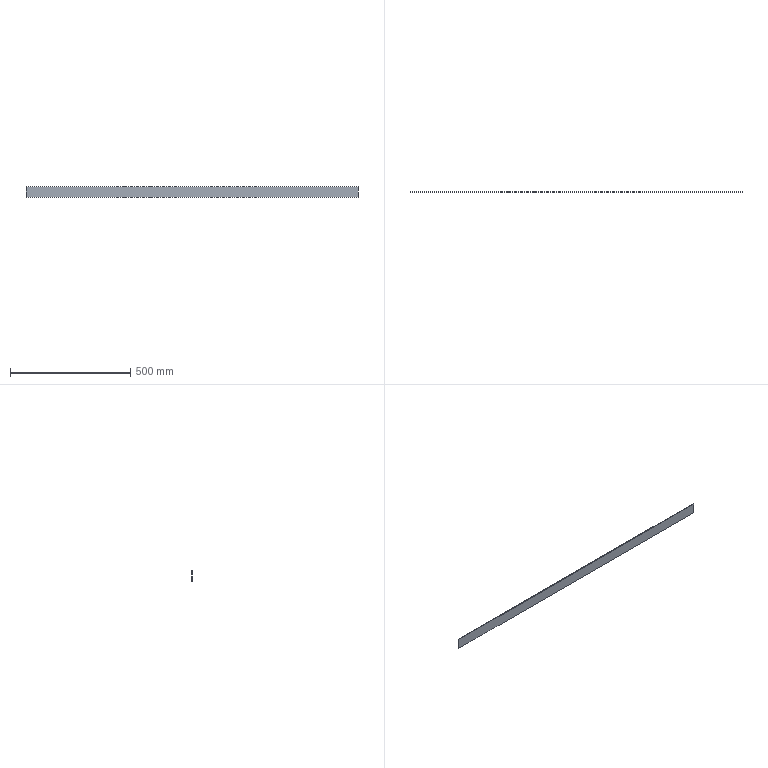Part | STEP file | SN10_017_002-01_CHAPA | 1 solid | 6 faces | box 1382 x 3 x 45 mm | volume 186570 mm3 | plane 6
STEP:
#1=CARTESIAN_POINT('',(0.,0.,0.));
#2=DIRECTION('',(0.,0.,1.));
#3=DIRECTION('',(1.,0.,0.));
#4=AXIS2_PLACEMENT_3D('',#1,#2,#3);
#5=CARTESIAN_POINT('',(3520.,-1740.,50.));
#6=VERTEX_POINT('',#5);
#7=CARTESIAN_POINT('',(2138.,-1740.,50.));
#8=VERTEX_POINT('',#7);
#9=CARTESIAN_POINT('',(3520.,-1740.,50.));
#10=DIRECTION('',(-1.,0.,0.));
#11=VECTOR('',#10,1.);
#12=LINE('',#9,#11);
#13=CARTESIAN_POINT('',(3520.,-1740.,95.));
#14=DIRECTION('',(0.,-1.,0.));
#15=DIRECTION('',(0.,0.,-1.));
#16=AXIS2_PLACEMENT_3D('',#13,#14,#15);
#17=PLANE('',#16);
#18=CARTESIAN_POINT('',(45.,0.));
#19=DIRECTION('',(0.,-1.));
#20=VECTOR('',#19,1.);
#21=LINE('',#18,#20);
#22=(GEOMETRIC_REPRESENTATION_CONTEXT(2)PARAMETRIC_REPRESENTATION_CONTEXT()REPRESENTATION_CONTEXT('',''));
#23=DEFINITIONAL_REPRESENTATION('',(#21),#22);
#24=PCURVE('',#17,#23);
#25=CARTESIAN_POINT('',(0.,0.,50.));
#26=DIRECTION('',(0.,0.,1.));
#27=DIRECTION('',(1.,0.,0.));
#28=AXIS2_PLACEMENT_3D('',#25,#26,#27);
#29=PLANE('',#28);
#30=CARTESIAN_POINT('',(3520.,-1740.));
#31=DIRECTION('',(-1.,0.));
#32=VECTOR('',#31,1.);
#33=LINE('',#30,#32);
#34=(GEOMETRIC_REPRESENTATION_CONTEXT(2)PARAMETRIC_REPRESENTATION_CONTEXT()REPRESENTATION_CONTEXT('',''));
#35=DEFINITIONAL_REPRESENTATION('',(#33),#34);
#36=PCURVE('',#29,#35);
#37=SURFACE_CURVE('',#12,(#24,#36),.PCURVE_S1.);
#38=EDGE_CURVE('',#6,#8,#37,.T.);
#39=ORIENTED_EDGE('',*,*,#38,.T.);
#40=CARTESIAN_POINT('',(2138.,-1740.,95.));
#41=VERTEX_POINT('',#40);
#42=CARTESIAN_POINT('',(2138.,-1740.,95.));
#43=DIRECTION('',(0.,0.,-1.));
#44=VECTOR('',#43,1.);
#45=LINE('',#42,#44);
#46=CARTESIAN_POINT('',(0.,-1382.));
#47=DIRECTION('',(1.,0.));
#48=VECTOR('',#47,1.);
#49=LINE('',#46,#48);
#50=(GEOMETRIC_REPRESENTATION_CONTEXT(2)PARAMETRIC_REPRESENTATION_CONTEXT()REPRESENTATION_CONTEXT('',''));
#51=DEFINITIONAL_REPRESENTATION('',(#49),#50);
#52=PCURVE('',#17,#51);
#53=CARTESIAN_POINT('',(2138.,-1740.,95.));
#54=DIRECTION('',(1.,0.,0.));
#55=DIRECTION('',(0.,0.,-1.));
#56=AXIS2_PLACEMENT_3D('',#53,#54,#55);
#57=PLANE('',#56);
#58=CARTESIAN_POINT('',(0.,0.));
#59=DIRECTION('',(1.,0.));
#60=VECTOR('',#59,1.);
#61=LINE('',#58,#60);
#62=(GEOMETRIC_REPRESENTATION_CONTEXT(2)PARAMETRIC_REPRESENTATION_CONTEXT()REPRESENTATION_CONTEXT('',''));
#63=DEFINITIONAL_REPRESENTATION('',(#61),#62);
#64=PCURVE('',#57,#63);
#65=SURFACE_CURVE('',#45,(#52,#64),.PCURVE_S1.);
#66=EDGE_CURVE('',#41,#8,#65,.T.);
#67=ORIENTED_EDGE('',*,*,#66,.F.);
#68=CARTESIAN_POINT('',(3520.,-1740.,95.));
#69=VERTEX_POINT('',#68);
#70=CARTESIAN_POINT('',(3520.,-1740.,95.));
#71=DIRECTION('',(-1.,0.,0.));
#72=VECTOR('',#71,1.);
#73=LINE('',#70,#72);
#74=CARTESIAN_POINT('',(0.,0.));
#75=DIRECTION('',(0.,-1.));
#76=VECTOR('',#75,1.);
#77=LINE('',#74,#76);
#78=(GEOMETRIC_REPRESENTATION_CONTEXT(2)PARAMETRIC_REPRESENTATION_CONTEXT()REPRESENTATION_CONTEXT('',''));
#79=DEFINITIONAL_REPRESENTATION('',(#77),#78);
#80=PCURVE('',#17,#79);
#81=CARTESIAN_POINT('',(0.,0.,95.));
#82=DIRECTION('',(0.,0.,1.));
#83=DIRECTION('',(1.,0.,0.));
#84=AXIS2_PLACEMENT_3D('',#81,#82,#83);
#85=PLANE('',#84);
#86=CARTESIAN_POINT('',(3520.,-1740.));
#87=DIRECTION('',(-1.,0.));
#88=VECTOR('',#87,1.);
#89=LINE('',#86,#88);
#90=(GEOMETRIC_REPRESENTATION_CONTEXT(2)PARAMETRIC_REPRESENTATION_CONTEXT()REPRESENTATION_CONTEXT('',''));
#91=DEFINITIONAL_REPRESENTATION('',(#89),#90);
#92=PCURVE('',#85,#91);
#93=SURFACE_CURVE('',#73,(#80,#92),.PCURVE_S1.);
#94=EDGE_CURVE('',#69,#41,#93,.T.);
#95=ORIENTED_EDGE('',*,*,#94,.F.);
#96=CARTESIAN_POINT('',(3520.,-1740.,95.));
#97=DIRECTION('',(0.,0.,-1.));
#98=VECTOR('',#97,1.);
#99=LINE('',#96,#98);
#100=CARTESIAN_POINT('',(0.,0.));
#101=DIRECTION('',(1.,0.));
#102=VECTOR('',#101,1.);
#103=LINE('',#100,#102);
#104=(GEOMETRIC_REPRESENTATION_CONTEXT(2)PARAMETRIC_REPRESENTATION_CONTEXT()REPRESENTATION_CONTEXT('',''));
#105=DEFINITIONAL_REPRESENTATION('',(#103),#104);
#106=PCURVE('',#17,#105);
#107=CARTESIAN_POINT('',(3520.,-1743.,95.));
#108=DIRECTION('',(-1.,0.,0.));
#109=DIRECTION('',(0.,0.,1.));
#110=AXIS2_PLACEMENT_3D('',#107,#108,#109);
#111=PLANE('',#110);
#112=CARTESIAN_POINT('',(0.,3.));
#113=DIRECTION('',(-1.,0.));
#114=VECTOR('',#113,1.);
#115=LINE('',#112,#114);
#116=(GEOMETRIC_REPRESENTATION_CONTEXT(2)PARAMETRIC_REPRESENTATION_CONTEXT()REPRESENTATION_CONTEXT('',''));
#117=DEFINITIONAL_REPRESENTATION('',(#115),#116);
#118=PCURVE('',#111,#117);
#119=SURFACE_CURVE('',#99,(#106,#118),.PCURVE_S1.);
#120=EDGE_CURVE('',#69,#6,#119,.T.);
#121=ORIENTED_EDGE('',*,*,#120,.T.);
#122=EDGE_LOOP('',(#39,#67,#95,#121));
#123=FACE_BOUND('',#122,.T.);
#124=ADVANCED_FACE('',(#123),#17,.F.);
#125=CARTESIAN_POINT('',(2138.,-1743.,50.));
#126=VERTEX_POINT('',#125);
#127=CARTESIAN_POINT('',(2138.,-1740.,50.));
#128=DIRECTION('',(0.,-1.,0.));
#129=VECTOR('',#128,1.);
#130=LINE('',#127,#129);
#131=CARTESIAN_POINT('',(45.,0.));
#132=DIRECTION('',(0.,-1.));
#133=VECTOR('',#132,1.);
#134=LINE('',#131,#133);
#135=(GEOMETRIC_REPRESENTATION_CONTEXT(2)PARAMETRIC_REPRESENTATION_CONTEXT()REPRESENTATION_CONTEXT('',''));
#136=DEFINITIONAL_REPRESENTATION('',(#134),#135);
#137=PCURVE('',#57,#136);
#138=CARTESIAN_POINT('',(2138.,-1740.));
#139=DIRECTION('',(0.,-1.));
#140=VECTOR('',#139,1.);
#141=LINE('',#138,#140);
#142=(GEOMETRIC_REPRESENTATION_CONTEXT(2)PARAMETRIC_REPRESENTATION_CONTEXT()REPRESENTATION_CONTEXT('',''));
#143=DEFINITIONAL_REPRESENTATION('',(#141),#142);
#144=PCURVE('',#29,#143);
#145=SURFACE_CURVE('',#130,(#137,#144),.PCURVE_S1.);
#146=EDGE_CURVE('',#8,#126,#145,.T.);
#147=ORIENTED_EDGE('',*,*,#146,.T.);
#148=CARTESIAN_POINT('',(2138.,-1743.,95.));
#149=VERTEX_POINT('',#148);
#150=CARTESIAN_POINT('',(2138.,-1743.,95.));
#151=DIRECTION('',(0.,0.,-1.));
#152=VECTOR('',#151,1.);
#153=LINE('',#150,#152);
#154=CARTESIAN_POINT('',(0.,-3.));
#155=DIRECTION('',(1.,0.));
#156=VECTOR('',#155,1.);
#157=LINE('',#154,#156);
#158=(GEOMETRIC_REPRESENTATION_CONTEXT(2)PARAMETRIC_REPRESENTATION_CONTEXT()REPRESENTATION_CONTEXT('',''));
#159=DEFINITIONAL_REPRESENTATION('',(#157),#158);
#160=PCURVE('',#57,#159);
#161=CARTESIAN_POINT('',(3520.,-1743.,95.));
#162=DIRECTION('',(0.,-1.,0.));
#163=DIRECTION('',(0.,0.,-1.));
#164=AXIS2_PLACEMENT_3D('',#161,#162,#163);
#165=PLANE('',#164);
#166=CARTESIAN_POINT('',(0.,-1382.));
#167=DIRECTION('',(1.,0.));
#168=VECTOR('',#167,1.);
#169=LINE('',#166,#168);
#170=(GEOMETRIC_REPRESENTATION_CONTEXT(2)PARAMETRIC_REPRESENTATION_CONTEXT()REPRESENTATION_CONTEXT('',''));
#171=DEFINITIONAL_REPRESENTATION('',(#169),#170);
#172=PCURVE('',#165,#171);
#173=SURFACE_CURVE('',#153,(#160,#172),.PCURVE_S1.);
#174=EDGE_CURVE('',#149,#126,#173,.T.);
#175=ORIENTED_EDGE('',*,*,#174,.F.);
#176=CARTESIAN_POINT('',(2138.,-1740.,95.));
#177=DIRECTION('',(0.,-1.,0.));
#178=VECTOR('',#177,1.);
#179=LINE('',#176,#178);
#180=CARTESIAN_POINT('',(0.,0.));
#181=DIRECTION('',(0.,-1.));
#182=VECTOR('',#181,1.);
#183=LINE('',#180,#182);
#184=(GEOMETRIC_REPRESENTATION_CONTEXT(2)PARAMETRIC_REPRESENTATION_CONTEXT()REPRESENTATION_CONTEXT('',''));
#185=DEFINITIONAL_REPRESENTATION('',(#183),#184);
#186=PCURVE('',#57,#185);
#187=CARTESIAN_POINT('',(2138.,-1740.));
#188=DIRECTION('',(0.,-1.));
#189=VECTOR('',#188,1.);
#190=LINE('',#187,#189);
#191=(GEOMETRIC_REPRESENTATION_CONTEXT(2)PARAMETRIC_REPRESENTATION_CONTEXT()REPRESENTATION_CONTEXT('',''));
#192=DEFINITIONAL_REPRESENTATION('',(#190),#191);
#193=PCURVE('',#85,#192);
#194=SURFACE_CURVE('',#179,(#186,#193),.PCURVE_S1.);
#195=EDGE_CURVE('',#41,#149,#194,.T.);
#196=ORIENTED_EDGE('',*,*,#195,.F.);
#197=ORIENTED_EDGE('',*,*,#66,.T.);
#198=EDGE_LOOP('',(#147,#175,#196,#197));
#199=FACE_BOUND('',#198,.T.);
#200=ADVANCED_FACE('',(#199),#57,.F.);
#201=CARTESIAN_POINT('',(3520.,-1743.,95.));
#202=VERTEX_POINT('',#201);
#203=CARTESIAN_POINT('',(3520.,-1743.,50.));
#204=VERTEX_POINT('',#203);
#205=CARTESIAN_POINT('',(3520.,-1743.,95.));
#206=DIRECTION('',(0.,0.,-1.));
#207=VECTOR('',#206,1.);
#208=LINE('',#205,#207);
#209=CARTESIAN_POINT('',(0.,0.));
#210=DIRECTION('',(1.,0.));
#211=VECTOR('',#210,1.);
#212=LINE('',#209,#211);
#213=(GEOMETRIC_REPRESENTATION_CONTEXT(2)PARAMETRIC_REPRESENTATION_CONTEXT()REPRESENTATION_CONTEXT('',''));
#214=DEFINITIONAL_REPRESENTATION('',(#212),#213);
#215=PCURVE('',#165,#214);
#216=CARTESIAN_POINT('',(0.,0.));
#217=DIRECTION('',(-1.,0.));
#218=VECTOR('',#217,1.);
#219=LINE('',#216,#218);
#220=(GEOMETRIC_REPRESENTATION_CONTEXT(2)PARAMETRIC_REPRESENTATION_CONTEXT()REPRESENTATION_CONTEXT('',''));
#221=DEFINITIONAL_REPRESENTATION('',(#219),#220);
#222=PCURVE('',#111,#221);
#223=SURFACE_CURVE('',#208,(#215,#222),.PCURVE_S1.);
#224=EDGE_CURVE('',#202,#204,#223,.T.);
#225=ORIENTED_EDGE('',*,*,#224,.F.);
#226=CARTESIAN_POINT('',(3520.,-1743.,95.));
#227=DIRECTION('',(-1.,0.,0.));
#228=VECTOR('',#227,1.);
#229=LINE('',#226,#228);
#230=CARTESIAN_POINT('',(0.,0.));
#231=DIRECTION('',(0.,-1.));
#232=VECTOR('',#231,1.);
#233=LINE('',#230,#232);
#234=(GEOMETRIC_REPRESENTATION_CONTEXT(2)PARAMETRIC_REPRESENTATION_CONTEXT()REPRESENTATION_CONTEXT('',''));
#235=DEFINITIONAL_REPRESENTATION('',(#233),#234);
#236=PCURVE('',#165,#235);
#237=CARTESIAN_POINT('',(3520.,-1743.));
#238=DIRECTION('',(-1.,0.));
#239=VECTOR('',#238,1.);
#240=LINE('',#237,#239);
#241=(GEOMETRIC_REPRESENTATION_CONTEXT(2)PARAMETRIC_REPRESENTATION_CONTEXT()REPRESENTATION_CONTEXT('',''));
#242=DEFINITIONAL_REPRESENTATION('',(#240),#241);
#243=PCURVE('',#85,#242);
#244=SURFACE_CURVE('',#229,(#236,#243),.PCURVE_S1.);
#245=EDGE_CURVE('',#202,#149,#244,.T.);
#246=ORIENTED_EDGE('',*,*,#245,.T.);
#247=ORIENTED_EDGE('',*,*,#174,.T.);
#248=CARTESIAN_POINT('',(3520.,-1743.,50.));
#249=DIRECTION('',(-1.,0.,0.));
#250=VECTOR('',#249,1.);
#251=LINE('',#248,#250);
#252=CARTESIAN_POINT('',(45.,0.));
#253=DIRECTION('',(0.,-1.));
#254=VECTOR('',#253,1.);
#255=LINE('',#252,#254);
#256=(GEOMETRIC_REPRESENTATION_CONTEXT(2)PARAMETRIC_REPRESENTATION_CONTEXT()REPRESENTATION_CONTEXT('',''));
#257=DEFINITIONAL_REPRESENTATION('',(#255),#256);
#258=PCURVE('',#165,#257);
#259=CARTESIAN_POINT('',(3520.,-1743.));
#260=DIRECTION('',(-1.,0.));
#261=VECTOR('',#260,1.);
#262=LINE('',#259,#261);
#263=(GEOMETRIC_REPRESENTATION_CONTEXT(2)PARAMETRIC_REPRESENTATION_CONTEXT()REPRESENTATION_CONTEXT('',''));
#264=DEFINITIONAL_REPRESENTATION('',(#262),#263);
#265=PCURVE('',#29,#264);
#266=SURFACE_CURVE('',#251,(#258,#265),.PCURVE_S1.);
#267=EDGE_CURVE('',#204,#126,#266,.T.);
#268=ORIENTED_EDGE('',*,*,#267,.F.);
#269=EDGE_LOOP('',(#225,#246,#247,#268));
#270=FACE_BOUND('',#269,.T.);
#271=ADVANCED_FACE('',(#270),#165,.T.);
#272=CARTESIAN_POINT('',(3520.,-1743.,50.));
#273=DIRECTION('',(0.,1.,0.));
#274=VECTOR('',#273,1.);
#275=LINE('',#272,#274);
#276=CARTESIAN_POINT('',(-45.,0.));
#277=DIRECTION('',(0.,1.));
#278=VECTOR('',#277,1.);
#279=LINE('',#276,#278);
#280=(GEOMETRIC_REPRESENTATION_CONTEXT(2)PARAMETRIC_REPRESENTATION_CONTEXT()REPRESENTATION_CONTEXT('',''));
#281=DEFINITIONAL_REPRESENTATION('',(#279),#280);
#282=PCURVE('',#111,#281);
#283=CARTESIAN_POINT('',(3520.,-1743.));
#284=DIRECTION('',(0.,1.));
#285=VECTOR('',#284,1.);
#286=LINE('',#283,#285);
#287=(GEOMETRIC_REPRESENTATION_CONTEXT(2)PARAMETRIC_REPRESENTATION_CONTEXT()REPRESENTATION_CONTEXT('',''));
#288=DEFINITIONAL_REPRESENTATION('',(#286),#287);
#289=PCURVE('',#29,#288);
#290=SURFACE_CURVE('',#275,(#282,#289),.PCURVE_S1.);
#291=EDGE_CURVE('',#204,#6,#290,.T.);
#292=ORIENTED_EDGE('',*,*,#291,.T.);
#293=ORIENTED_EDGE('',*,*,#120,.F.);
#294=CARTESIAN_POINT('',(3520.,-1743.,95.));
#295=DIRECTION('',(0.,1.,0.));
#296=VECTOR('',#295,1.);
#297=LINE('',#294,#296);
#298=CARTESIAN_POINT('',(0.,0.));
#299=DIRECTION('',(0.,1.));
#300=VECTOR('',#299,1.);
#301=LINE('',#298,#300);
#302=(GEOMETRIC_REPRESENTATION_CONTEXT(2)PARAMETRIC_REPRESENTATION_CONTEXT()REPRESENTATION_CONTEXT('',''));
#303=DEFINITIONAL_REPRESENTATION('',(#301),#302);
#304=PCURVE('',#111,#303);
#305=CARTESIAN_POINT('',(3520.,-1743.));
#306=DIRECTION('',(0.,1.));
#307=VECTOR('',#306,1.);
#308=LINE('',#305,#307);
#309=(GEOMETRIC_REPRESENTATION_CONTEXT(2)PARAMETRIC_REPRESENTATION_CONTEXT()REPRESENTATION_CONTEXT('',''));
#310=DEFINITIONAL_REPRESENTATION('',(#308),#309);
#311=PCURVE('',#85,#310);
#312=SURFACE_CURVE('',#297,(#304,#311),.PCURVE_S1.);
#313=EDGE_CURVE('',#202,#69,#312,.T.);
#314=ORIENTED_EDGE('',*,*,#313,.F.);
#315=ORIENTED_EDGE('',*,*,#224,.T.);
#316=EDGE_LOOP('',(#292,#293,#314,#315));
#317=FACE_BOUND('',#316,.T.);
#318=ADVANCED_FACE('',(#317),#111,.F.);
#319=ORIENTED_EDGE('',*,*,#94,.T.);
#320=ORIENTED_EDGE('',*,*,#195,.T.);
#321=ORIENTED_EDGE('',*,*,#245,.F.);
#322=ORIENTED_EDGE('',*,*,#313,.T.);
#323=EDGE_LOOP('',(#319,#320,#321,#322));
#324=FACE_BOUND('',#323,.T.);
#325=ADVANCED_FACE('',(#324),#85,.T.);
#326=ORIENTED_EDGE('',*,*,#291,.F.);
#327=ORIENTED_EDGE('',*,*,#267,.T.);
#328=ORIENTED_EDGE('',*,*,#146,.F.);
#329=ORIENTED_EDGE('',*,*,#38,.F.);
#330=EDGE_LOOP('',(#326,#327,#328,#329));
#331=FACE_BOUND('',#330,.T.);
#332=ADVANCED_FACE('',(#331),#29,.F.);
#333=CLOSED_SHELL('',(#124,#200,#271,#318,#325,#332));
#334=MANIFOLD_SOLID_BREP('',#333);
#335=(LENGTH_UNIT()NAMED_UNIT(*)SI_UNIT(.MILLI.,.METRE.));
#336=UNCERTAINTY_MEASURE_WITH_UNIT(LENGTH_MEASURE(0.0000001),#335,'','');
#337=(NAMED_UNIT(*)PLANE_ANGLE_UNIT()SI_UNIT($,.RADIAN.));
#338=(NAMED_UNIT(*)SI_UNIT($,.STERADIAN.)SOLID_ANGLE_UNIT());
#339=(GEOMETRIC_REPRESENTATION_CONTEXT(3)GLOBAL_UNCERTAINTY_ASSIGNED_CONTEXT((#336))GLOBAL_UNIT_ASSIGNED_CONTEXT((#335,#337,#338))REPRESENTATION_CONTEXT('',''));
#340=ADVANCED_BREP_SHAPE_REPRESENTATION('',(#4,#334),#339);